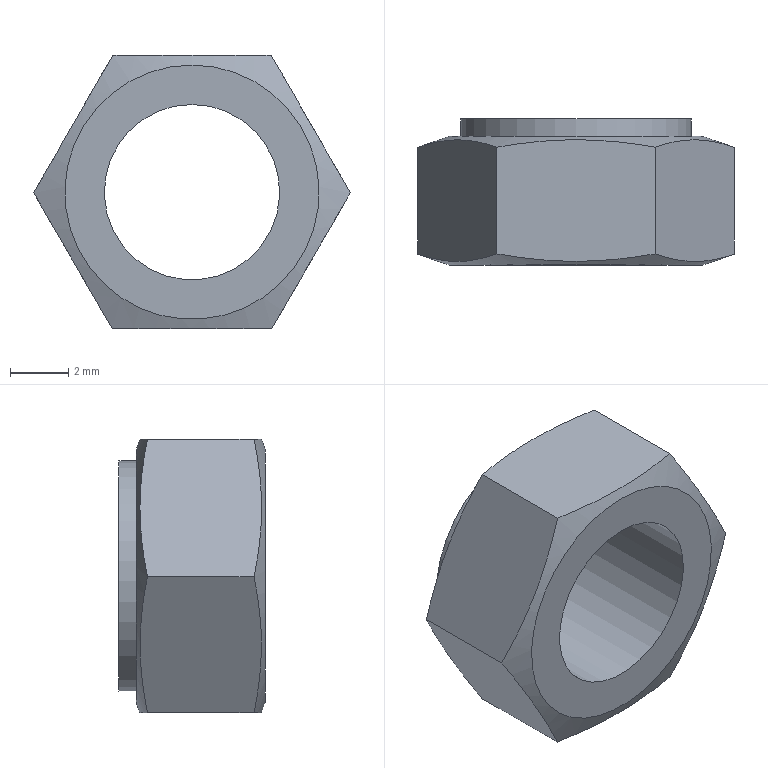Part | STEP file | GB13681-1992 nut M6 | 1 solid | 13 faces | box 10.835 x 5 x 9.372 mm | volume 219.571 mm3 | plane 9 | cylinder 2 | cone 2 | commonest cylinder face diameters 6 x1 7.9 x1
STEP:
#1=CARTESIAN_POINT('',(0.,0.,3.));
#2=VERTEX_POINT('',#1);
#3=CARTESIAN_POINT('',(0.,0.,0.));
#4=DIRECTION('',(0.,1.,0.));
#5=DIRECTION('',(0.,0.,1.));
#6=AXIS2_PLACEMENT_3D('',#3,#4,#5);
#7=CIRCLE('',#6,3.);
#8=EDGE_CURVE('',#2,#2,#7,.T.);
#9=ORIENTED_EDGE('',*,*,#8,.F.);
#10=EDGE_LOOP('',(#9));
#11=FACE_OUTER_BOUND('',#10,.T.);
#12=CARTESIAN_POINT('',(0.,5.,3.));
#13=VERTEX_POINT('',#12);
#14=CARTESIAN_POINT('',(0.,5.,0.));
#15=DIRECTION('',(0.,1.,0.));
#16=DIRECTION('',(0.,0.,1.));
#17=AXIS2_PLACEMENT_3D('',#14,#15,#16);
#18=CIRCLE('',#17,3.);
#19=EDGE_CURVE('',#13,#13,#18,.T.);
#20=ORIENTED_EDGE('',*,*,#19,.T.);
#21=EDGE_LOOP('',(#20));
#22=FACE_OUTER_BOUND('',#21,.T.);
#23=CARTESIAN_POINT('',(0.,6.4,0.));
#24=DIRECTION('',(0.,1.,0.));
#25=DIRECTION('',(0.,0.,1.));
#26=AXIS2_PLACEMENT_3D('',#23,#24,#25);
#27=CYLINDRICAL_SURFACE('',#26,3.);
#28=ADVANCED_FACE('',(#11,#22),#27,.F.);
#29=CARTESIAN_POINT('',(0.,0.,4.35));
#30=VERTEX_POINT('',#29);
#31=CARTESIAN_POINT('',(0.,0.,0.));
#32=DIRECTION('',(0.,1.,0.));
#33=DIRECTION('',(0.,0.,1.));
#34=AXIS2_PLACEMENT_3D('',#31,#32,#33);
#35=CIRCLE('',#34,4.35);
#36=EDGE_CURVE('',#30,#30,#35,.T.);
#37=ORIENTED_EDGE('',*,*,#36,.F.);
#38=EDGE_LOOP('',(#37));
#39=FACE_OUTER_BOUND('',#38,.T.);
#40=ORIENTED_EDGE('',*,*,#8,.T.);
#41=EDGE_LOOP('',(#40));
#42=FACE_BOUND('',#41,.T.);
#43=CARTESIAN_POINT('',(3.,0.,0.));
#44=DIRECTION('',(0.,1.,0.));
#45=DIRECTION('',(0.,0.,1.));
#46=AXIS2_PLACEMENT_3D('',#43,#44,#45);
#47=PLANE('',#46);
#48=ADVANCED_FACE('',(#39,#42),#47,.F.);
#49=CARTESIAN_POINT('',(2.729,0.375,-4.68));
#50=VERTEX_POINT('',#49);
#51=CARTESIAN_POINT('',(5.418,0.375,-0.0233));
#52=VERTEX_POINT('',#51);
#53=CARTESIAN_POINT('',(2.729,0.375,-4.68));
#54=CARTESIAN_POINT('',(3.177,0.2188,-3.904));
#55=CARTESIAN_POINT('',(4.073,0.02955,-2.352));
#56=CARTESIAN_POINT('',(4.97,0.2188,-0.7994));
#57=CARTESIAN_POINT('',(5.418,0.375,-0.0233));
#58=B_SPLINE_CURVE_WITH_KNOTS('',3,(#53,#54,#55,#56,#57),.UNSPECIFIED.,.F.,.F.,(4,1,4),(0.000000231,0.002689,0.005377),.UNSPECIFIED.);
#59=EDGE_CURVE('',#50,#52,#58,.T.);
#60=ORIENTED_EDGE('',*,*,#59,.T.);
#61=CARTESIAN_POINT('',(2.709,0.375,4.692));
#62=VERTEX_POINT('',#61);
#63=CARTESIAN_POINT('',(5.418,0.375,-0.0233));
#64=CARTESIAN_POINT('',(4.966,0.2153,0.7626));
#65=CARTESIAN_POINT('',(4.063,0.02082,2.334));
#66=CARTESIAN_POINT('',(3.16,0.2153,3.906));
#67=CARTESIAN_POINT('',(2.709,0.375,4.692));
#68=B_SPLINE_CURVE_WITH_KNOTS('',3,(#63,#64,#65,#66,#67),.UNSPECIFIED.,.F.,.F.,(4,1,4),(0.000000231,0.002719,0.005438),.UNSPECIFIED.);
#69=EDGE_CURVE('',#52,#62,#68,.T.);
#70=ORIENTED_EDGE('',*,*,#69,.T.);
#71=CARTESIAN_POINT('',(-2.709,0.375,4.692));
#72=VERTEX_POINT('',#71);
#73=CARTESIAN_POINT('',(2.709,0.375,4.692));
#74=CARTESIAN_POINT('',(1.81,0.2171,4.692));
#75=CARTESIAN_POINT('',(0.9085,0.1204,4.692));
#76=CARTESIAN_POINT('',(-0.4467,0.1199,4.692));
#77=CARTESIAN_POINT('',(-0.8991,0.1431,4.692));
#78=CARTESIAN_POINT('',(-1.805,0.2312,4.692));
#79=CARTESIAN_POINT('',(-2.259,0.296,4.692));
#80=CARTESIAN_POINT('',(-2.709,0.375,4.692));
#81=B_SPLINE_CURVE_WITH_KNOTS('',3,(#73,#74,#75,#76,#77,#78,#79,#80),.UNSPECIFIED.,.F.,.F.,(4,2,2,4),(0.009965,0.01269,0.01406,0.01542),.UNSPECIFIED.);
#82=EDGE_CURVE('',#62,#72,#81,.T.);
#83=ORIENTED_EDGE('',*,*,#82,.T.);
#84=CARTESIAN_POINT('',(-5.418,0.375,-0.02341));
#85=VERTEX_POINT('',#84);
#86=CARTESIAN_POINT('',(-2.709,0.375,4.692));
#87=CARTESIAN_POINT('',(-3.16,0.2153,3.906));
#88=CARTESIAN_POINT('',(-4.063,0.02081,2.334));
#89=CARTESIAN_POINT('',(-4.966,0.2153,0.7625));
#90=CARTESIAN_POINT('',(-5.418,0.375,-0.02341));
#91=B_SPLINE_CURVE_WITH_KNOTS('',3,(#86,#87,#88,#89,#90),.UNSPECIFIED.,.F.,.F.,(4,1,4),(0.000000231,0.002719,0.005438),.UNSPECIFIED.);
#92=EDGE_CURVE('',#72,#85,#91,.T.);
#93=ORIENTED_EDGE('',*,*,#92,.T.);
#94=CARTESIAN_POINT('',(-2.729,0.375,-4.68));
#95=VERTEX_POINT('',#94);
#96=CARTESIAN_POINT('',(-5.418,0.375,-0.02341));
#97=CARTESIAN_POINT('',(-4.97,0.2188,-0.7995));
#98=CARTESIAN_POINT('',(-4.073,0.02956,-2.352));
#99=CARTESIAN_POINT('',(-3.177,0.2188,-3.904));
#100=CARTESIAN_POINT('',(-2.729,0.375,-4.68));
#101=B_SPLINE_CURVE_WITH_KNOTS('',3,(#96,#97,#98,#99,#100),.UNSPECIFIED.,.F.,.F.,(4,1,4),(0.000000231,0.002689,0.005377),.UNSPECIFIED.);
#102=EDGE_CURVE('',#85,#95,#101,.T.);
#103=ORIENTED_EDGE('',*,*,#102,.T.);
#104=CARTESIAN_POINT('',(-2.729,0.375,-4.68));
#105=CARTESIAN_POINT('',(-2.276,0.2949,-4.68));
#106=CARTESIAN_POINT('',(-1.819,0.2289,-4.68));
#107=CARTESIAN_POINT('',(-0.906,0.1394,-4.68));
#108=CARTESIAN_POINT('',(-0.4503,0.1158,-4.68));
#109=CARTESIAN_POINT('',(0.9151,0.1163,-4.68));
#110=CARTESIAN_POINT('',(1.823,0.2147,-4.68));
#111=CARTESIAN_POINT('',(2.729,0.375,-4.68));
#112=B_SPLINE_CURVE_WITH_KNOTS('',3,(#104,#105,#106,#107,#108,#109,#110,#111),.UNSPECIFIED.,.F.,.F.,(4,2,2,4),(0.004575,0.005953,0.00733,0.01009),.UNSPECIFIED.);
#113=EDGE_CURVE('',#95,#50,#112,.T.);
#114=ORIENTED_EDGE('',*,*,#113,.T.);
#115=EDGE_LOOP('',(#60,#70,#83,#93,#103,#114));
#116=FACE_OUTER_BOUND('',#115,.T.);
#117=ORIENTED_EDGE('',*,*,#36,.T.);
#118=EDGE_LOOP('',(#117));
#119=FACE_BOUND('',#118,.T.);
#120=CARTESIAN_POINT('',(0.,0.,0.));
#121=DIRECTION('',(0.,1.,0.));
#122=DIRECTION('',(0.,0.,1.));
#123=AXIS2_PLACEMENT_3D('',#120,#121,#122);
#124=CONICAL_SURFACE('',#123,4.35,1.233);
#125=ADVANCED_FACE('',(#116,#119),#124,.T.);
#126=CARTESIAN_POINT('',(0.,4.4,4.35));
#127=VERTEX_POINT('',#126);
#128=CARTESIAN_POINT('',(0.,4.4,0.));
#129=DIRECTION('',(0.,1.,0.));
#130=DIRECTION('',(0.,0.,1.));
#131=AXIS2_PLACEMENT_3D('',#128,#129,#130);
#132=CIRCLE('',#131,4.35);
#133=EDGE_CURVE('',#127,#127,#132,.T.);
#134=ORIENTED_EDGE('',*,*,#133,.F.);
#135=EDGE_LOOP('',(#134));
#136=FACE_BOUND('',#135,.T.);
#137=CARTESIAN_POINT('',(-2.709,4.025,4.692));
#138=VERTEX_POINT('',#137);
#139=CARTESIAN_POINT('',(2.709,4.025,4.692));
#140=VERTEX_POINT('',#139);
#141=CARTESIAN_POINT('',(-2.709,4.025,4.692));
#142=CARTESIAN_POINT('',(-2.259,4.104,4.692));
#143=CARTESIAN_POINT('',(-1.805,4.169,4.692));
#144=CARTESIAN_POINT('',(-0.8991,4.257,4.692));
#145=CARTESIAN_POINT('',(-0.4467,4.28,4.692));
#146=CARTESIAN_POINT('',(0.9085,4.28,4.692));
#147=CARTESIAN_POINT('',(1.81,4.183,4.692));
#148=CARTESIAN_POINT('',(2.709,4.025,4.692));
#149=B_SPLINE_CURVE_WITH_KNOTS('',3,(#141,#142,#143,#144,#145,#146,#147,#148),.UNSPECIFIED.,.F.,.F.,(4,2,2,4),(0.004585,0.005953,0.00732,0.01005),.UNSPECIFIED.);
#150=EDGE_CURVE('',#138,#140,#149,.T.);
#151=ORIENTED_EDGE('',*,*,#150,.T.);
#152=CARTESIAN_POINT('',(5.418,4.025,-0.0233));
#153=VERTEX_POINT('',#152);
#154=CARTESIAN_POINT('',(2.709,4.025,4.692));
#155=CARTESIAN_POINT('',(3.16,4.185,3.906));
#156=CARTESIAN_POINT('',(4.063,4.379,2.334));
#157=CARTESIAN_POINT('',(4.966,4.185,0.7626));
#158=CARTESIAN_POINT('',(5.418,4.025,-0.0233));
#159=B_SPLINE_CURVE_WITH_KNOTS('',3,(#154,#155,#156,#157,#158),.UNSPECIFIED.,.F.,.F.,(4,1,4),(0.000000231,0.002719,0.005438),.UNSPECIFIED.);
#160=EDGE_CURVE('',#140,#153,#159,.T.);
#161=ORIENTED_EDGE('',*,*,#160,.T.);
#162=CARTESIAN_POINT('',(2.729,4.025,-4.68));
#163=VERTEX_POINT('',#162);
#164=CARTESIAN_POINT('',(5.418,4.025,-0.0233));
#165=CARTESIAN_POINT('',(4.97,4.181,-0.7994));
#166=CARTESIAN_POINT('',(4.073,4.37,-2.352));
#167=CARTESIAN_POINT('',(3.177,4.181,-3.904));
#168=CARTESIAN_POINT('',(2.729,4.025,-4.68));
#169=B_SPLINE_CURVE_WITH_KNOTS('',3,(#164,#165,#166,#167,#168),.UNSPECIFIED.,.F.,.F.,(4,1,4),(0.000000231,0.002689,0.005377),.UNSPECIFIED.);
#170=EDGE_CURVE('',#153,#163,#169,.T.);
#171=ORIENTED_EDGE('',*,*,#170,.T.);
#172=CARTESIAN_POINT('',(-2.729,4.025,-4.68));
#173=VERTEX_POINT('',#172);
#174=CARTESIAN_POINT('',(2.729,4.025,-4.68));
#175=CARTESIAN_POINT('',(1.823,4.185,-4.68));
#176=CARTESIAN_POINT('',(0.9151,4.284,-4.68));
#177=CARTESIAN_POINT('',(-0.4503,4.284,-4.68));
#178=CARTESIAN_POINT('',(-0.906,4.261,-4.68));
#179=CARTESIAN_POINT('',(-1.819,4.171,-4.68));
#180=CARTESIAN_POINT('',(-2.276,4.105,-4.68));
#181=CARTESIAN_POINT('',(-2.729,4.025,-4.68));
#182=B_SPLINE_CURVE_WITH_KNOTS('',3,(#174,#175,#176,#177,#178,#179,#180,#181),.UNSPECIFIED.,.F.,.F.,(4,2,2,4),(0.009999,0.01275,0.01412,0.0155),.UNSPECIFIED.);
#183=EDGE_CURVE('',#163,#173,#182,.T.);
#184=ORIENTED_EDGE('',*,*,#183,.T.);
#185=CARTESIAN_POINT('',(-5.418,4.025,-0.02341));
#186=VERTEX_POINT('',#185);
#187=CARTESIAN_POINT('',(-2.729,4.025,-4.68));
#188=CARTESIAN_POINT('',(-3.177,4.181,-3.904));
#189=CARTESIAN_POINT('',(-4.073,4.37,-2.352));
#190=CARTESIAN_POINT('',(-4.97,4.181,-0.7995));
#191=CARTESIAN_POINT('',(-5.418,4.025,-0.02341));
#192=B_SPLINE_CURVE_WITH_KNOTS('',3,(#187,#188,#189,#190,#191),.UNSPECIFIED.,.F.,.F.,(4,1,4),(0.000000231,0.002689,0.005377),.UNSPECIFIED.);
#193=EDGE_CURVE('',#173,#186,#192,.T.);
#194=ORIENTED_EDGE('',*,*,#193,.T.);
#195=CARTESIAN_POINT('',(-5.418,4.025,-0.02341));
#196=CARTESIAN_POINT('',(-4.966,4.185,0.7625));
#197=CARTESIAN_POINT('',(-4.063,4.379,2.334));
#198=CARTESIAN_POINT('',(-3.16,4.185,3.906));
#199=CARTESIAN_POINT('',(-2.709,4.025,4.692));
#200=B_SPLINE_CURVE_WITH_KNOTS('',3,(#195,#196,#197,#198,#199),.UNSPECIFIED.,.F.,.F.,(4,1,4),(0.000000231,0.002719,0.005438),.UNSPECIFIED.);
#201=EDGE_CURVE('',#186,#138,#200,.T.);
#202=ORIENTED_EDGE('',*,*,#201,.T.);
#203=EDGE_LOOP('',(#151,#161,#171,#184,#194,#202));
#204=FACE_OUTER_BOUND('',#203,.T.);
#205=CARTESIAN_POINT('',(0.,4.025,0.));
#206=DIRECTION('',(0.,-1.,0.));
#207=DIRECTION('',(0.,0.,-1.));
#208=AXIS2_PLACEMENT_3D('',#205,#206,#207);
#209=CONICAL_SURFACE('',#208,5.418,1.233);
#210=ADVANCED_FACE('',(#136,#204),#209,.T.);
#211=CARTESIAN_POINT('',(0.,4.4,3.95));
#212=VERTEX_POINT('',#211);
#213=CARTESIAN_POINT('',(0.,4.4,0.));
#214=DIRECTION('',(0.,1.,0.));
#215=DIRECTION('',(0.,0.,1.));
#216=AXIS2_PLACEMENT_3D('',#213,#214,#215);
#217=CIRCLE('',#216,3.95);
#218=EDGE_CURVE('',#212,#212,#217,.T.);
#219=ORIENTED_EDGE('',*,*,#218,.F.);
#220=EDGE_LOOP('',(#219));
#221=FACE_BOUND('',#220,.T.);
#222=ORIENTED_EDGE('',*,*,#133,.T.);
#223=EDGE_LOOP('',(#222));
#224=FACE_OUTER_BOUND('',#223,.T.);
#225=CARTESIAN_POINT('',(4.35,4.4,0.));
#226=DIRECTION('',(0.,-1.,0.));
#227=DIRECTION('',(0.,0.,-1.));
#228=AXIS2_PLACEMENT_3D('',#225,#226,#227);
#229=PLANE('',#228);
#230=ADVANCED_FACE('',(#221,#224),#229,.F.);
#231=CARTESIAN_POINT('',(0.,5.,3.95));
#232=VERTEX_POINT('',#231);
#233=CARTESIAN_POINT('',(0.,5.,0.));
#234=DIRECTION('',(0.,1.,0.));
#235=DIRECTION('',(0.,0.,1.));
#236=AXIS2_PLACEMENT_3D('',#233,#234,#235);
#237=CIRCLE('',#236,3.95);
#238=EDGE_CURVE('',#232,#232,#237,.T.);
#239=ORIENTED_EDGE('',*,*,#238,.F.);
#240=EDGE_LOOP('',(#239));
#241=FACE_OUTER_BOUND('',#240,.T.);
#242=ORIENTED_EDGE('',*,*,#218,.T.);
#243=EDGE_LOOP('',(#242));
#244=FACE_OUTER_BOUND('',#243,.T.);
#245=CARTESIAN_POINT('',(0.,6.4,0.));
#246=DIRECTION('',(0.,1.,0.));
#247=DIRECTION('',(0.,0.,1.));
#248=AXIS2_PLACEMENT_3D('',#245,#246,#247);
#249=CYLINDRICAL_SURFACE('',#248,3.95);
#250=ADVANCED_FACE('',(#241,#244),#249,.T.);
#251=ORIENTED_EDGE('',*,*,#19,.F.);
#252=EDGE_LOOP('',(#251));
#253=FACE_BOUND('',#252,.T.);
#254=ORIENTED_EDGE('',*,*,#238,.T.);
#255=EDGE_LOOP('',(#254));
#256=FACE_OUTER_BOUND('',#255,.T.);
#257=CARTESIAN_POINT('',(3.95,5.,0.));
#258=DIRECTION('',(0.,-1.,0.));
#259=DIRECTION('',(0.,0.,-1.));
#260=AXIS2_PLACEMENT_3D('',#257,#258,#259);
#261=PLANE('',#260);
#262=ADVANCED_FACE('',(#253,#256),#261,.F.);
#263=CARTESIAN_POINT('',(5.418,5.,-0.0233));
#264=DIRECTION('',(0.,-1.,0.));
#265=VECTOR('',#264,1000.);
#266=LINE('',#263,#265);
#267=EDGE_CURVE('',#153,#52,#266,.T.);
#268=ORIENTED_EDGE('',*,*,#267,.F.);
#269=ORIENTED_EDGE('',*,*,#160,.F.);
#270=CARTESIAN_POINT('',(2.709,5.,4.692));
#271=DIRECTION('',(0.,-1.,0.));
#272=VECTOR('',#271,1000.);
#273=LINE('',#270,#272);
#274=EDGE_CURVE('',#140,#62,#273,.T.);
#275=ORIENTED_EDGE('',*,*,#274,.T.);
#276=ORIENTED_EDGE('',*,*,#69,.F.);
#277=EDGE_LOOP('',(#268,#269,#275,#276));
#278=FACE_OUTER_BOUND('',#277,.T.);
#279=CARTESIAN_POINT('',(2.709,5.,4.692));
#280=DIRECTION('',(-0.8671,0.,-0.4981));
#281=DIRECTION('',(-0.4981,0.,0.8671));
#282=AXIS2_PLACEMENT_3D('',#279,#280,#281);
#283=PLANE('',#282);
#284=ADVANCED_FACE('',(#278),#283,.F.);
#285=CARTESIAN_POINT('',(2.729,5.,-4.68));
#286=DIRECTION('',(0.,-1.,0.));
#287=VECTOR('',#286,1000.);
#288=LINE('',#285,#287);
#289=EDGE_CURVE('',#163,#50,#288,.T.);
#290=ORIENTED_EDGE('',*,*,#289,.F.);
#291=ORIENTED_EDGE('',*,*,#170,.F.);
#292=ORIENTED_EDGE('',*,*,#267,.T.);
#293=ORIENTED_EDGE('',*,*,#59,.F.);
#294=EDGE_LOOP('',(#290,#291,#292,#293));
#295=FACE_OUTER_BOUND('',#294,.T.);
#296=CARTESIAN_POINT('',(5.418,5.,-0.0233));
#297=DIRECTION('',(-0.866,0.,0.5));
#298=DIRECTION('',(0.5,0.,0.866));
#299=AXIS2_PLACEMENT_3D('',#296,#297,#298);
#300=PLANE('',#299);
#301=ADVANCED_FACE('',(#295),#300,.F.);
#302=CARTESIAN_POINT('',(-2.729,5.,-4.68));
#303=DIRECTION('',(0.,-1.,0.));
#304=VECTOR('',#303,1000.);
#305=LINE('',#302,#304);
#306=EDGE_CURVE('',#173,#95,#305,.T.);
#307=ORIENTED_EDGE('',*,*,#306,.F.);
#308=ORIENTED_EDGE('',*,*,#183,.F.);
#309=ORIENTED_EDGE('',*,*,#289,.T.);
#310=ORIENTED_EDGE('',*,*,#113,.F.);
#311=EDGE_LOOP('',(#307,#308,#309,#310));
#312=FACE_OUTER_BOUND('',#311,.T.);
#313=CARTESIAN_POINT('',(2.729,5.,-4.68));
#314=DIRECTION('',(0.,0.,1.));
#315=DIRECTION('',(1.,0.,0.));
#316=AXIS2_PLACEMENT_3D('',#313,#314,#315);
#317=PLANE('',#316);
#318=ADVANCED_FACE('',(#312),#317,.F.);
#319=CARTESIAN_POINT('',(-5.418,5.,-0.02341));
#320=DIRECTION('',(0.,-1.,0.));
#321=VECTOR('',#320,1000.);
#322=LINE('',#319,#321);
#323=EDGE_CURVE('',#186,#85,#322,.T.);
#324=ORIENTED_EDGE('',*,*,#323,.F.);
#325=ORIENTED_EDGE('',*,*,#193,.F.);
#326=ORIENTED_EDGE('',*,*,#306,.T.);
#327=ORIENTED_EDGE('',*,*,#102,.F.);
#328=EDGE_LOOP('',(#324,#325,#326,#327));
#329=FACE_OUTER_BOUND('',#328,.T.);
#330=CARTESIAN_POINT('',(-2.729,5.,-4.68));
#331=DIRECTION('',(0.866,0.,0.5));
#332=DIRECTION('',(0.5,0.,-0.866));
#333=AXIS2_PLACEMENT_3D('',#330,#331,#332);
#334=PLANE('',#333);
#335=ADVANCED_FACE('',(#329),#334,.F.);
#336=CARTESIAN_POINT('',(-2.709,5.,4.692));
#337=DIRECTION('',(0.,-1.,0.));
#338=VECTOR('',#337,1000.);
#339=LINE('',#336,#338);
#340=EDGE_CURVE('',#138,#72,#339,.T.);
#341=ORIENTED_EDGE('',*,*,#340,.F.);
#342=ORIENTED_EDGE('',*,*,#201,.F.);
#343=ORIENTED_EDGE('',*,*,#323,.T.);
#344=ORIENTED_EDGE('',*,*,#92,.F.);
#345=EDGE_LOOP('',(#341,#342,#343,#344));
#346=FACE_OUTER_BOUND('',#345,.T.);
#347=CARTESIAN_POINT('',(-5.418,5.,-0.02341));
#348=DIRECTION('',(0.8671,0.,-0.4981));
#349=DIRECTION('',(-0.4981,0.,-0.8671));
#350=AXIS2_PLACEMENT_3D('',#347,#348,#349);
#351=PLANE('',#350);
#352=ADVANCED_FACE('',(#346),#351,.F.);
#353=ORIENTED_EDGE('',*,*,#274,.F.);
#354=ORIENTED_EDGE('',*,*,#150,.F.);
#355=ORIENTED_EDGE('',*,*,#340,.T.);
#356=ORIENTED_EDGE('',*,*,#82,.F.);
#357=EDGE_LOOP('',(#353,#354,#355,#356));
#358=FACE_OUTER_BOUND('',#357,.T.);
#359=CARTESIAN_POINT('',(-2.709,5.,4.692));
#360=DIRECTION('',(0.,0.,-1.));
#361=DIRECTION('',(-1.,0.,0.));
#362=AXIS2_PLACEMENT_3D('',#359,#360,#361);
#363=PLANE('',#362);
#364=ADVANCED_FACE('',(#358),#363,.F.);
#365=CLOSED_SHELL('',(#28,#48,#125,#210,#230,#250,#262,#284,#301,#318,#335,#352,#364));
#366=MANIFOLD_SOLID_BREP('',#365);
#367=CARTESIAN_POINT('',(0.,0.,0.));
#368=DIRECTION('',(0.,0.,1.));
#369=DIRECTION('',(1.,0.,0.));
#370=AXIS2_PLACEMENT_3D('',#367,#368,#369);
#371=(LENGTH_UNIT()NAMED_UNIT(*)SI_UNIT(.MILLI.,.METRE.));
#372=UNCERTAINTY_MEASURE_WITH_UNIT(LENGTH_MEASURE(0.00001),#371,'','');
#373=(NAMED_UNIT(*)PLANE_ANGLE_UNIT()SI_UNIT($,.RADIAN.));
#374=(NAMED_UNIT(*)SI_UNIT($,.STERADIAN.)SOLID_ANGLE_UNIT());
#375=(GEOMETRIC_REPRESENTATION_CONTEXT(3)GLOBAL_UNCERTAINTY_ASSIGNED_CONTEXT((#372))GLOBAL_UNIT_ASSIGNED_CONTEXT((#371,#373,#374))REPRESENTATION_CONTEXT('',''));
#376=ADVANCED_BREP_SHAPE_REPRESENTATION('',(#366,#370),#375);